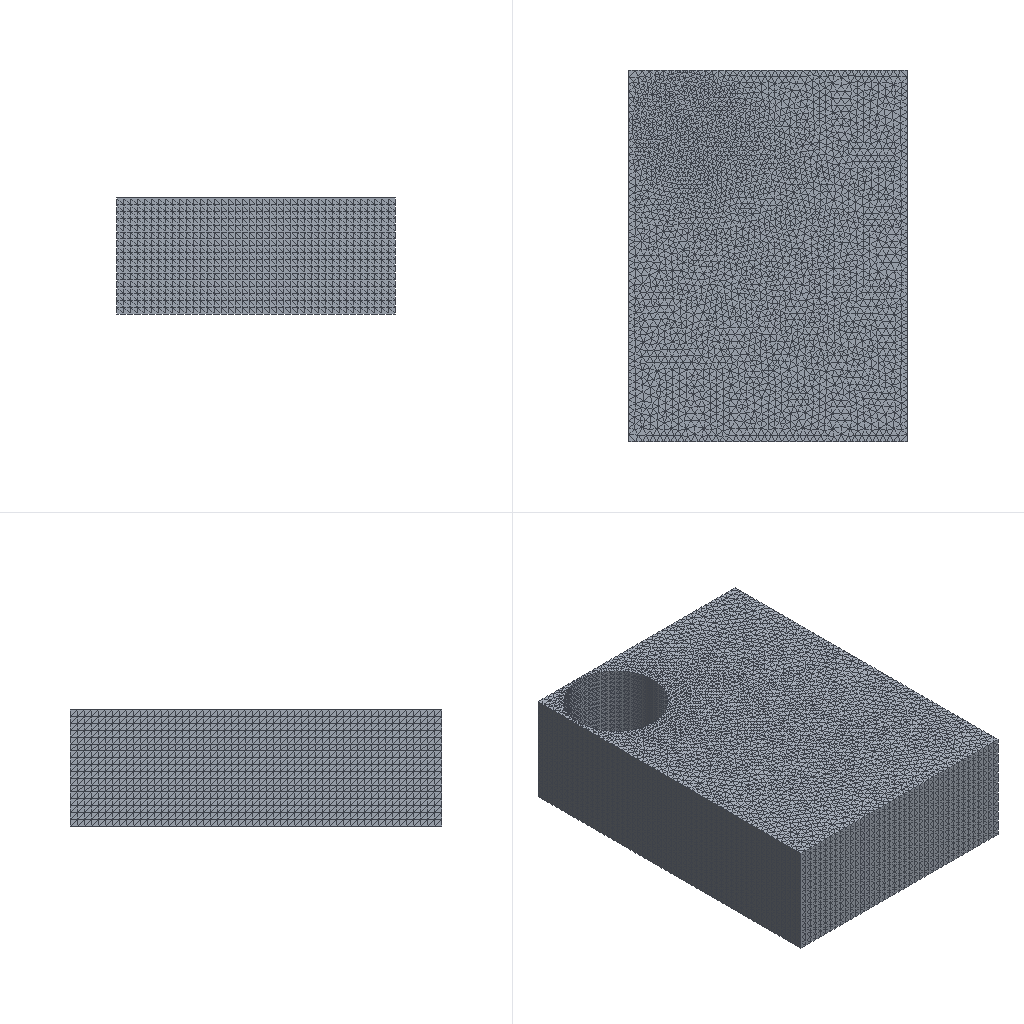Simulation study | abaqus
Set-up summary:
category,name,step,type,value,unit,region
solver,abaqus
solver,version,,,Abaqus/Explicit 2020
units,not stated in the deck,,not stated
analysis,deck,,transient,transient
load_step,Step-1,Step-1,transient
load_step,requested,,,1
mesh,nodes,,,42365
mesh,elements,,,210107
element_type,C3D4,,solid,201965
element_type,R3D3,,rigid,8142
load,load commands in deck,,count,3
bc,support commands in deck,,count,7
material,MATERIAL-1,,in results
check,setup vs results,,match,"per instance, exact: element labels, types and connectivity; labels of the nodes the elements use; coordinates of those nodes at SINGLE_PRECISION in 2 of 2 instance(s)"
Abaqus input file, long lists of numbers shortened:
*Heading
** Job name: Job-2 Model name: Model-1
** Generated by: Abaqus/CAE 2020
*Preprint, echo=NO, model=NO, history=NO, contact=NO
**
** PARTS
**
*Part, name=daojiu
*Node
      1,           3.,           0.,         -35.
      2,           3.,           0.,         -20.
** (4065 more lines like these left out)
*Element, type=R3D3
 1,    1,  644, 2335
 2, 2335, 2342,    1
** (8140 more lines like these left out)
*Node
   4068, 4.36618125e-15, -3.55271368e-15,  -59.35
*Nset, nset=daojiu-RefPt_, internal
4068,
*Elset, elset=daojiu, generate
    1,  8142,     1
*End Part
**
*Part, name=gongjian
*Node
      1,         -60.,          90.,           0.
      2,          60.,          90.,           0.
** (38295 more lines like these left out)
*Element, type=C3D4
     1,  9579,  9580,  9581,  9582
     2,  9583,  9584,  9582,  9579
** (201963 more lines like these left out)
*Nset, nset=Set-4, generate
     1,  38297,      1
*Elset, elset=Set-4, generate
      1,  201965,       1
** Section: Section-1
*Solid Section, elset=Set-4, material=Material-1
,
*End Part
**
**
** ASSEMBLY
**
*Assembly, name=Assembly
**
*Instance, name=daojiu-1, part=daojiu
        -36.,         66.5,    70.35
*End Instance
**
*Instance, name=gongjian-1, part=gongjian
*End Instance
**
*Nset, nset=Set-1, instance=gongjian-1
    1,    2,    3,    4,   13,   14,   15,   16,   17,   18,   19,   20,   21,   22,   23,   24
   25,   26,   27,   28,   29,   30,   31,   32,   33,   34,   35,   36,   37,   38,   39,   40
** (137 more lines like these left out)
*Elset, elset=Set-1, instance=gongjian-1
    379,    905,   1065,   1568,   1606,   1821,   1911,   2725,   3323,   3403,   3615,   3777,   4043,   4776,   6390,   6456
   7045,   7619,   7762,   7857,   8162,   8186,   8534,   8776,   8889,   8980,   9236,   9293,   9444,   9484,   9502,  10297
** (263 more lines like these left out)
*Nset, nset=Set-2, instance=daojiu-1
 4068,
*Nset, nset=Set-4, instance=daojiu-1
 4068,
*Nset, nset=s_Set-3, instance=gongjian-1, generate
     1,  38297,      1
*Elset, elset=s_Set-3, instance=gongjian-1, generate
      1,  201965,       1
*Elset, elset=_m_Surf-1_SPOS, internal, instance=daojiu-1, generate
 3148,  3233,     1
*Surface, type=ELEMENT, name=m_Surf-1
_m_Surf-1_SPOS, SPOS
*Elset, elset=_m_Surf-2_SPOS, internal, instance=daojiu-1, generate
 2588,  2673,     1
*Surface, type=ELEMENT, name=m_Surf-2
_m_Surf-2_SPOS, SPOS
*Elset, elset=_m_Surf-3_SPOS, internal, instance=daojiu-1, generate
 2028,  2113,     1
*Surface, type=ELEMENT, name=m_Surf-3
_m_Surf-3_SPOS, SPOS
*Elset, elset=_m_Surf-4_SPOS, internal, instance=daojiu-1, generate
 3760,  3845,     1
*Surface, type=ELEMENT, name=m_Surf-4
_m_Surf-4_SPOS, SPOS
*Elset, elset=_m_Surf-5_SPOS, internal, instance=daojiu-1
  901,  902,  903,  904,  905,  906,  907,  908,  909,  910,  911,  912,  913,  914,  915,  916
  917,  918,  919,  920,  921,  922,  923,  924,  925,  926,  927,  928,  929,  930,  931,  932
** (8 more lines like these left out)
*Surface, type=ELEMENT, name=m_Surf-5
_m_Surf-5_SPOS, SPOS
*Elset, elset=_m_Surf-6_SPOS, internal, instance=daojiu-1
  633,  634,  635,  636,  637,  638,  639,  640,  641,  642,  643,  644,  645,  646,  647,  648
  649,  650,  651,  652,  653,  654,  655,  656,  657,  658,  659,  660,  661,  662,  663,  664
** (8 more lines like these left out)
*Surface, type=ELEMENT, name=m_Surf-6
_m_Surf-6_SPOS, SPOS
*Elset, elset=_m_Surf-7_SPOS, internal, instance=daojiu-1
  365,  366,  367,  368,  369,  370,  371,  372,  373,  374,  375,  376,  377,  378,  379,  380
  381,  382,  383,  384,  385,  386,  387,  388,  389,  390,  391,  392,  393,  394,  395,  396
** (8 more lines like these left out)
*Surface, type=ELEMENT, name=m_Surf-7
_m_Surf-7_SPOS, SPOS
*Elset, elset=_m_Surf-8_SPOS, internal, instance=daojiu-1
   97,   98,   99,  100,  101,  102,  103,  104,  105,  106,  107,  108,  109,  110,  111,  112
  113,  114,  115,  116,  117,  118,  119,  120,  121,  122,  123,  124,  125,  126,  127,  128
** (8 more lines like these left out)
*Surface, type=ELEMENT, name=m_Surf-8
_m_Surf-8_SPOS, SPOS
*Elset, elset=_m_Surf-9_SPOS, internal, instance=daojiu-1
 1169, 1170, 1171, 1172, 1173, 1174, 1175, 1176, 1177, 1178, 1179, 1180, 1181, 1182, 1183, 1184
 1185, 1186, 1187, 1188, 1189, 1190, 1191, 1192, 1193, 1194, 1195, 1196, 1197, 1198, 1199, 1200
** (147 more lines like these left out)
*Surface, type=ELEMENT, name=m_Surf-9
_m_Surf-9_SPOS, SPOS
*Surface, type=NODE, name=s_Set-3_CNS_, internal
s_Set-3, 1.
*Rigid Body, ref node=daojiu-1.daojiu-RefPt_, elset=daojiu-1.daojiu
*End Assembly
*Amplitude, name=Amp-1, definition=PERIODIC
1,           1256.,              0.,              0.
             1.,              0.
**
** MATERIALS
**
*Material, name=Material-1
*Damage Initiation, criterion=JOHNSON COOK
 -0.09,  0.25,  -0.5, 0.014,  3.87, 1650.,   25.,    1.
*Damage Evolution, type=DISPLACEMENT
 1e-05,
*Density
 4.4e-09,
*Elastic
108000., 0.33
*Plastic, hardening=JOHNSON COOK
860., 683., 0.47,   1.,1650.,  25.
*Rate Dependent, type=JOHNSON COOK
 0.035,1.
**
** INTERACTION PROPERTIES
**
*Surface Interaction, name=IntProp-1
*Friction
 0.15,
*Surface Behavior, pressure-overclosure=HARD
** ----------------------------------------------------------------
**
** STEP: Step-1
**
*Step, name=Step-1, nlgeom=YES
*Dynamic, Explicit
, 0.1
*Bulk Viscosity
0.06, 1.2
** Mass Scaling: Semi-Automatic
**               Whole Model
*Fixed Mass Scaling, factor=500.
**
** BOUNDARY CONDITIONS
**
** Name: BC-1 Type: 对称/反对称/完全固定
*Boundary
Set-1, ENCASTRE
** Name: [REDACTED]
*Boundary, amplitude=Amp-1
Set-4, 3, 3, -20.
** Name: [REDACTED] : Velocity/Angular velocity
*Boundary, type=VELOCITY
Set-2, 1, 1
Set-2, 2, 2, -1200.
Set-2, 4, 4
Set-2, 5, 5
Set-2, 6, 6, -400.
**
** INTERACTIONS
**
** Interaction: Int-2
*Contact Pair, interaction=IntProp-1, mechanical constraint=KINEMATIC, cpset=Int-2
m_Surf-1, s_Set-3_CNS_
** Interaction: Int-2-Copy
*Contact Pair, interaction=IntProp-1, mechanical constraint=KINEMATIC, cpset=Int-2-Copy
m_Surf-3, s_Set-3_CNS_
** Interaction: Int-3
*Contact Pair, interaction=IntProp-1, mechanical constraint=KINEMATIC, cpset=Int-3
m_Surf-2, s_Set-3_CNS_
** Interaction: Int-3-Copy
*Contact Pair, interaction=IntProp-1, mechanical constraint=KINEMATIC, cpset=Int-3-Copy
m_Surf-4, s_Set-3_CNS_
** Interaction: Int-4
*Contact Pair, interaction=IntProp-1, mechanical constraint=KINEMATIC, cpset=Int-4
m_Surf-5, s_Set-3_CNS_
** Interaction: Int-4-Copy
*Contact Pair, interaction=IntProp-1, mechanical constraint=KINEMATIC, cpset=Int-4-Copy
m_Surf-6, s_Set-3_CNS_
** Interaction: Int-4-Copy2
*Contact Pair, interaction=IntProp-1, mechanical constraint=KINEMATIC, cpset=Int-4-Copy2
m_Surf-7, s_Set-3_CNS_
** Interaction: Int-4-Copy3
*Contact Pair, interaction=IntProp-1, mechanical constraint=KINEMATIC, cpset=Int-4-Copy3
m_Surf-8, s_Set-3_CNS_
** Interaction: Int-5
*Contact Pair, interaction=IntProp-1, mechanical constraint=KINEMATIC, cpset=Int-5
m_Surf-9, s_Set-3_CNS_
** Interaction: Int-9
*Contact, op=NEW
*Contact Inclusions, ALL EXTERIOR
*Contact Property Assignment
 ,  , IntProp-1
**
** OUTPUT REQUESTS
**
*Restart, write, number interval=1, time marks=NO
**
** FIELD OUTPUT: F-Output-1
**
*Output, field, number interval=50
*Node Output
A, CF, RF, RM, RT, U, V
*Element Output, directions=YES
E, EVF, LE, MISES, MISESMAX, PE, PEEQ, PEEQVAVG, PEVAVG, S, STATUS, SVAVG
*Contact Output
CDISP, CSTRESS
**
** HISTORY OUTPUT: H-Output-1
**
*Output, history, time interval=2e-06
*Node Output, nset=Set-2
RF1, RF2, RF3
*End Step
Results summary:
result,step,Step-1,partial,increments=1 time=0.0/0.1
result,analysis,,,transient
result,last_loadstep,,,1
result,primary field,,,U
result,reaction total,,FX,0.0,model units
result,reaction total,,FY,0.0,model units
result,reaction total,,FZ,0.0,model units